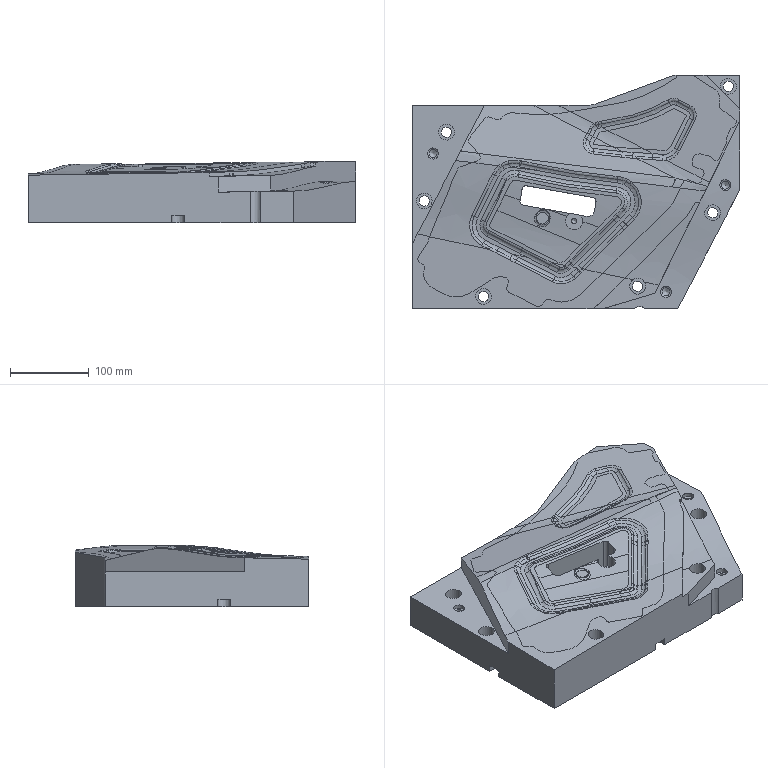Part | STEP file | gslz 2016.10.28-13_id1418_x_t | 1 solid | 253 faces | box 415 x 296 x 77.793 mm | volume 6493168 mm3 | spline 166 | plane 45 | cylinder 35 | cone 7 | commonest cylinder face diameters 13 x6 16 x6 20 x6 10 x4 10.3 x3 14 x3